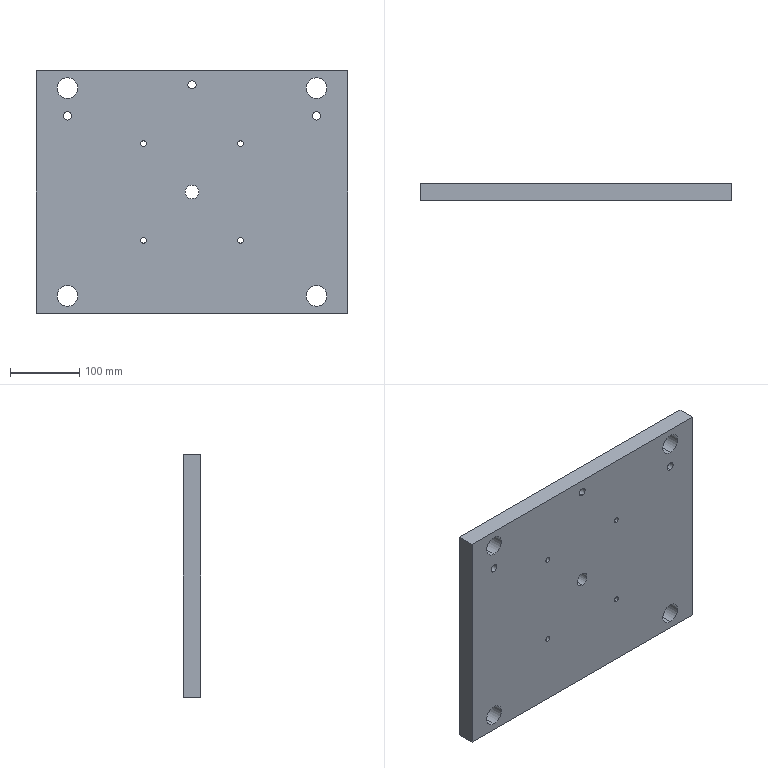Part | STEP file | OP10-101_base plate lower (R) | 1 solid | 30 faces | box 450 x 25 x 350 mm | volume 3845451 mm3 | cylinder 24 | plane 6 | commonest cylinder face diameters 8 x8 30 x8 12 x6 20 x2